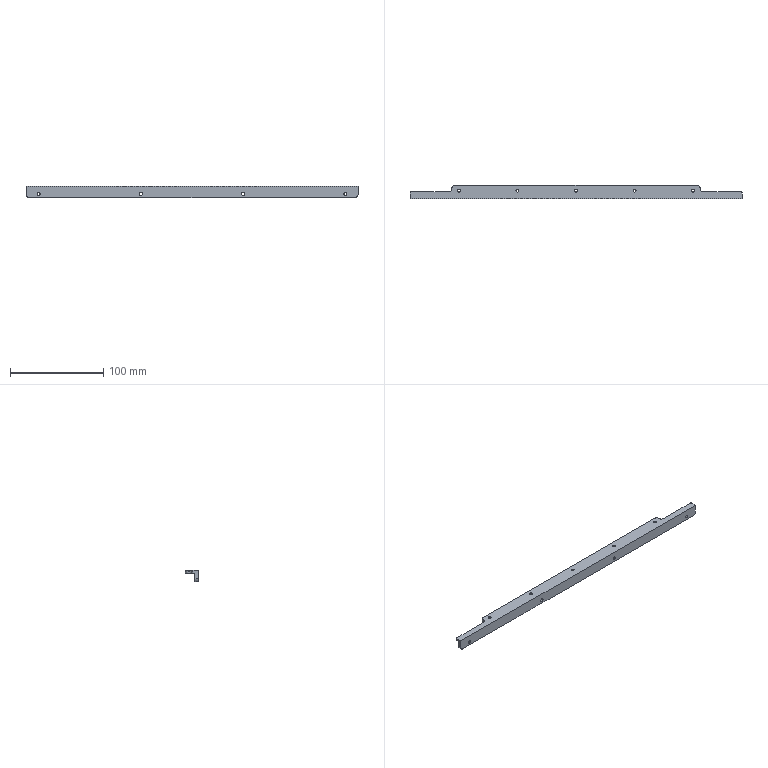Part | 1 solid | 48 faces | box 356.96 x 14 x 12 mm | volume 25600 mm3 | cylinder 26 | plane 12 | cone 10 | commonest cylinder face diameters 3.2 x10 3.3 x8 6 x6 2 x2
STEP:
#1=CARTESIAN_POINT('',(165.,4.,-6.35));
#2=VERTEX_POINT('',#1);
#3=CARTESIAN_POINT('',(165.,0.,-6.35));
#4=VERTEX_POINT('',#3);
#5=CARTESIAN_POINT('',(165.,0.,-6.35));
#6=DIRECTION('',(0.,-1.,0.));
#7=VECTOR('',#6,1000.);
#8=LINE('',#5,#7);
#9=EDGE_CURVE('',#2,#4,#8,.T.);
#10=ORIENTED_EDGE('',*,*,#9,.F.);
#11=CARTESIAN_POINT('',(165.,4.,-9.65));
#12=VERTEX_POINT('',#11);
#13=CARTESIAN_POINT('',(165.,4.,-8.));
#14=DIRECTION('',(0.,-1.,0.));
#15=DIRECTION('',(0.,0.,-1.));
#16=AXIS2_PLACEMENT_3D('',#13,#14,#15);
#17=CIRCLE('',#16,1.65);
#18=EDGE_CURVE('',#12,#2,#17,.T.);
#19=ORIENTED_EDGE('',*,*,#18,.F.);
#20=CARTESIAN_POINT('',(165.,0.,-9.65));
#21=VERTEX_POINT('',#20);
#22=CARTESIAN_POINT('',(165.,0.,-9.65));
#23=DIRECTION('',(0.,-1.,0.));
#24=VECTOR('',#23,1000.);
#25=LINE('',#22,#24);
#26=EDGE_CURVE('',#12,#21,#25,.T.);
#27=ORIENTED_EDGE('',*,*,#26,.T.);
#28=CARTESIAN_POINT('',(165.,0.,-8.));
#29=DIRECTION('',(0.,-1.,0.));
#30=DIRECTION('',(0.,0.,-1.));
#31=AXIS2_PLACEMENT_3D('',#28,#29,#30);
#32=CIRCLE('',#31,1.65);
#33=EDGE_CURVE('',#21,#4,#32,.T.);
#34=ORIENTED_EDGE('',*,*,#33,.T.);
#35=EDGE_LOOP('',(#10,#19,#27,#34));
#36=FACE_BOUND('',#35,.T.);
#37=CARTESIAN_POINT('',(165.,0.,-8.));
#38=DIRECTION('',(0.,-1.,0.));
#39=DIRECTION('',(0.,0.,-1.));
#40=AXIS2_PLACEMENT_3D('',#37,#38,#39);
#41=CYLINDRICAL_SURFACE('',#40,1.65);
#42=ADVANCED_FACE('',(#36),#41,.F.);
#43=CARTESIAN_POINT('',(55.,4.,-6.35));
#44=VERTEX_POINT('',#43);
#45=CARTESIAN_POINT('',(55.,0.,-6.35));
#46=VERTEX_POINT('',#45);
#47=CARTESIAN_POINT('',(55.,0.,-6.35));
#48=DIRECTION('',(0.,-1.,0.));
#49=VECTOR('',#48,1000.);
#50=LINE('',#47,#49);
#51=EDGE_CURVE('',#44,#46,#50,.T.);
#52=ORIENTED_EDGE('',*,*,#51,.F.);
#53=CARTESIAN_POINT('',(55.,4.,-9.65));
#54=VERTEX_POINT('',#53);
#55=CARTESIAN_POINT('',(55.,4.,-8.));
#56=DIRECTION('',(0.,-1.,0.));
#57=DIRECTION('',(0.,0.,-1.));
#58=AXIS2_PLACEMENT_3D('',#55,#56,#57);
#59=CIRCLE('',#58,1.65);
#60=EDGE_CURVE('',#54,#44,#59,.T.);
#61=ORIENTED_EDGE('',*,*,#60,.F.);
#62=CARTESIAN_POINT('',(55.,0.,-9.65));
#63=VERTEX_POINT('',#62);
#64=CARTESIAN_POINT('',(55.,0.,-9.65));
#65=DIRECTION('',(0.,-1.,0.));
#66=VECTOR('',#65,1000.);
#67=LINE('',#64,#66);
#68=EDGE_CURVE('',#54,#63,#67,.T.);
#69=ORIENTED_EDGE('',*,*,#68,.T.);
#70=CARTESIAN_POINT('',(55.,0.,-8.));
#71=DIRECTION('',(0.,-1.,0.));
#72=DIRECTION('',(0.,0.,-1.));
#73=AXIS2_PLACEMENT_3D('',#70,#71,#72);
#74=CIRCLE('',#73,1.65);
#75=EDGE_CURVE('',#63,#46,#74,.T.);
#76=ORIENTED_EDGE('',*,*,#75,.T.);
#77=EDGE_LOOP('',(#52,#61,#69,#76));
#78=FACE_BOUND('',#77,.T.);
#79=CARTESIAN_POINT('',(55.,0.,-8.));
#80=DIRECTION('',(0.,-1.,0.));
#81=DIRECTION('',(0.,0.,-1.));
#82=AXIS2_PLACEMENT_3D('',#79,#80,#81);
#83=CYLINDRICAL_SURFACE('',#82,1.65);
#84=ADVANCED_FACE('',(#78),#83,.F.);
#85=CARTESIAN_POINT('',(-55.,4.,-6.35));
#86=VERTEX_POINT('',#85);
#87=CARTESIAN_POINT('',(-55.,0.,-6.35));
#88=VERTEX_POINT('',#87);
#89=CARTESIAN_POINT('',(-55.,0.,-6.35));
#90=DIRECTION('',(0.,-1.,0.));
#91=VECTOR('',#90,1000.);
#92=LINE('',#89,#91);
#93=EDGE_CURVE('',#86,#88,#92,.T.);
#94=ORIENTED_EDGE('',*,*,#93,.F.);
#95=CARTESIAN_POINT('',(-55.,4.,-9.65));
#96=VERTEX_POINT('',#95);
#97=CARTESIAN_POINT('',(-55.,4.,-8.));
#98=DIRECTION('',(0.,-1.,0.));
#99=DIRECTION('',(0.,0.,-1.));
#100=AXIS2_PLACEMENT_3D('',#97,#98,#99);
#101=CIRCLE('',#100,1.65);
#102=EDGE_CURVE('',#96,#86,#101,.T.);
#103=ORIENTED_EDGE('',*,*,#102,.F.);
#104=CARTESIAN_POINT('',(-55.,0.,-9.65));
#105=VERTEX_POINT('',#104);
#106=CARTESIAN_POINT('',(-55.,0.,-9.65));
#107=DIRECTION('',(0.,-1.,0.));
#108=VECTOR('',#107,1000.);
#109=LINE('',#106,#108);
#110=EDGE_CURVE('',#96,#105,#109,.T.);
#111=ORIENTED_EDGE('',*,*,#110,.T.);
#112=CARTESIAN_POINT('',(-55.,0.,-8.));
#113=DIRECTION('',(0.,-1.,0.));
#114=DIRECTION('',(0.,0.,-1.));
#115=AXIS2_PLACEMENT_3D('',#112,#113,#114);
#116=CIRCLE('',#115,1.65);
#117=EDGE_CURVE('',#105,#88,#116,.T.);
#118=ORIENTED_EDGE('',*,*,#117,.T.);
#119=EDGE_LOOP('',(#94,#103,#111,#118));
#120=FACE_BOUND('',#119,.T.);
#121=CARTESIAN_POINT('',(-55.,0.,-8.));
#122=DIRECTION('',(0.,-1.,0.));
#123=DIRECTION('',(0.,0.,-1.));
#124=AXIS2_PLACEMENT_3D('',#121,#122,#123);
#125=CYLINDRICAL_SURFACE('',#124,1.65);
#126=ADVANCED_FACE('',(#120),#125,.F.);
#127=CARTESIAN_POINT('',(-165.,4.,-6.35));
#128=VERTEX_POINT('',#127);
#129=CARTESIAN_POINT('',(-165.,0.,-6.35));
#130=VERTEX_POINT('',#129);
#131=CARTESIAN_POINT('',(-165.,0.,-6.35));
#132=DIRECTION('',(0.,-1.,0.));
#133=VECTOR('',#132,1000.);
#134=LINE('',#131,#133);
#135=EDGE_CURVE('',#128,#130,#134,.T.);
#136=ORIENTED_EDGE('',*,*,#135,.F.);
#137=CARTESIAN_POINT('',(-165.,4.,-9.65));
#138=VERTEX_POINT('',#137);
#139=CARTESIAN_POINT('',(-165.,4.,-8.));
#140=DIRECTION('',(0.,-1.,0.));
#141=DIRECTION('',(0.,0.,-1.));
#142=AXIS2_PLACEMENT_3D('',#139,#140,#141);
#143=CIRCLE('',#142,1.65);
#144=EDGE_CURVE('',#138,#128,#143,.T.);
#145=ORIENTED_EDGE('',*,*,#144,.F.);
#146=CARTESIAN_POINT('',(-165.,0.,-9.65));
#147=VERTEX_POINT('',#146);
#148=CARTESIAN_POINT('',(-165.,0.,-9.65));
#149=DIRECTION('',(0.,-1.,0.));
#150=VECTOR('',#149,1000.);
#151=LINE('',#148,#150);
#152=EDGE_CURVE('',#138,#147,#151,.T.);
#153=ORIENTED_EDGE('',*,*,#152,.T.);
#154=CARTESIAN_POINT('',(-165.,0.,-8.));
#155=DIRECTION('',(0.,-1.,0.));
#156=DIRECTION('',(0.,0.,-1.));
#157=AXIS2_PLACEMENT_3D('',#154,#155,#156);
#158=CIRCLE('',#157,1.65);
#159=EDGE_CURVE('',#147,#130,#158,.T.);
#160=ORIENTED_EDGE('',*,*,#159,.T.);
#161=EDGE_LOOP('',(#136,#145,#153,#160));
#162=FACE_BOUND('',#161,.T.);
#163=CARTESIAN_POINT('',(-165.,0.,-8.));
#164=DIRECTION('',(0.,-1.,0.));
#165=DIRECTION('',(0.,0.,-1.));
#166=AXIS2_PLACEMENT_3D('',#163,#164,#165);
#167=CYLINDRICAL_SURFACE('',#166,1.65);
#168=ADVANCED_FACE('',(#162),#167,.F.);
#169=CARTESIAN_POINT('',(126.,6.9,-1.45));
#170=VERTEX_POINT('',#169);
#171=CARTESIAN_POINT('',(126.,5.35,-3.));
#172=VERTEX_POINT('',#171);
#173=CARTESIAN_POINT('',(126.,5.35,-3.));
#174=DIRECTION('',(0.,-0.7071,-0.7071));
#175=VECTOR('',#174,1000.);
#176=LINE('',#173,#175);
#177=EDGE_CURVE('',#170,#172,#176,.T.);
#178=ORIENTED_EDGE('',*,*,#177,.F.);
#179=CARTESIAN_POINT('',(126.,10.1,-1.45));
#180=VERTEX_POINT('',#179);
#181=CARTESIAN_POINT('',(126.,8.5,-1.45));
#182=DIRECTION('',(0.,0.,-1.));
#183=DIRECTION('',(0.,1.,0.));
#184=AXIS2_PLACEMENT_3D('',#181,#182,#183);
#185=CIRCLE('',#184,1.6);
#186=EDGE_CURVE('',#180,#170,#185,.T.);
#187=ORIENTED_EDGE('',*,*,#186,.F.);
#188=CARTESIAN_POINT('',(126.,11.65,-3.));
#189=VERTEX_POINT('',#188);
#190=CARTESIAN_POINT('',(126.,11.65,-3.));
#191=DIRECTION('',(0.,0.7071,-0.7071));
#192=VECTOR('',#191,1000.);
#193=LINE('',#190,#192);
#194=EDGE_CURVE('',#180,#189,#193,.T.);
#195=ORIENTED_EDGE('',*,*,#194,.T.);
#196=CARTESIAN_POINT('',(126.,8.5,-3.));
#197=DIRECTION('',(0.,0.,-1.));
#198=DIRECTION('',(0.,1.,0.));
#199=AXIS2_PLACEMENT_3D('',#196,#197,#198);
#200=CIRCLE('',#199,3.15);
#201=EDGE_CURVE('',#189,#172,#200,.T.);
#202=ORIENTED_EDGE('',*,*,#201,.T.);
#203=EDGE_LOOP('',(#178,#187,#195,#202));
#204=FACE_BOUND('',#203,.T.);
#205=CARTESIAN_POINT('',(126.,8.5,-3.));
#206=DIRECTION('',(0.,0.,-1.));
#207=DIRECTION('',(0.,1.,0.));
#208=AXIS2_PLACEMENT_3D('',#205,#206,#207);
#209=CONICAL_SURFACE('',#208,3.15,0.7854);
#210=ADVANCED_FACE('',(#204),#209,.F.);
#211=CARTESIAN_POINT('',(126.,6.9,0.));
#212=VERTEX_POINT('',#211);
#213=CARTESIAN_POINT('',(126.,6.9,-3.));
#214=DIRECTION('',(0.,0.,-1.));
#215=VECTOR('',#214,1000.);
#216=LINE('',#213,#215);
#217=EDGE_CURVE('',#212,#170,#216,.T.);
#218=ORIENTED_EDGE('',*,*,#217,.F.);
#219=CARTESIAN_POINT('',(126.,10.1,0.));
#220=VERTEX_POINT('',#219);
#221=CARTESIAN_POINT('',(126.,8.5,0.));
#222=DIRECTION('',(0.,0.,-1.));
#223=DIRECTION('',(-1.,0.,0.));
#224=AXIS2_PLACEMENT_3D('',#221,#222,#223);
#225=CIRCLE('',#224,1.6);
#226=EDGE_CURVE('',#220,#212,#225,.T.);
#227=ORIENTED_EDGE('',*,*,#226,.F.);
#228=CARTESIAN_POINT('',(126.,10.1,-3.));
#229=DIRECTION('',(0.,0.,-1.));
#230=VECTOR('',#229,1000.);
#231=LINE('',#228,#230);
#232=EDGE_CURVE('',#220,#180,#231,.T.);
#233=ORIENTED_EDGE('',*,*,#232,.T.);
#234=ORIENTED_EDGE('',*,*,#186,.T.);
#235=EDGE_LOOP('',(#218,#227,#233,#234));
#236=FACE_BOUND('',#235,.T.);
#237=CARTESIAN_POINT('',(126.,8.5,-3.));
#238=DIRECTION('',(0.,0.,-1.));
#239=DIRECTION('',(0.,1.,0.));
#240=AXIS2_PLACEMENT_3D('',#237,#238,#239);
#241=CYLINDRICAL_SURFACE('',#240,1.6);
#242=ADVANCED_FACE('',(#236),#241,.F.);
#243=CARTESIAN_POINT('',(63.,6.9,-1.45));
#244=VERTEX_POINT('',#243);
#245=CARTESIAN_POINT('',(63.,5.35,-3.));
#246=VERTEX_POINT('',#245);
#247=CARTESIAN_POINT('',(63.,5.35,-3.));
#248=DIRECTION('',(0.,-0.7071,-0.7071));
#249=VECTOR('',#248,1000.);
#250=LINE('',#247,#249);
#251=EDGE_CURVE('',#244,#246,#250,.T.);
#252=ORIENTED_EDGE('',*,*,#251,.F.);
#253=CARTESIAN_POINT('',(63.,10.1,-1.45));
#254=VERTEX_POINT('',#253);
#255=CARTESIAN_POINT('',(63.,8.5,-1.45));
#256=DIRECTION('',(0.,0.,-1.));
#257=DIRECTION('',(0.,1.,0.));
#258=AXIS2_PLACEMENT_3D('',#255,#256,#257);
#259=CIRCLE('',#258,1.6);
#260=EDGE_CURVE('',#254,#244,#259,.T.);
#261=ORIENTED_EDGE('',*,*,#260,.F.);
#262=CARTESIAN_POINT('',(63.,11.65,-3.));
#263=VERTEX_POINT('',#262);
#264=CARTESIAN_POINT('',(63.,11.65,-3.));
#265=DIRECTION('',(0.,0.7071,-0.7071));
#266=VECTOR('',#265,1000.);
#267=LINE('',#264,#266);
#268=EDGE_CURVE('',#254,#263,#267,.T.);
#269=ORIENTED_EDGE('',*,*,#268,.T.);
#270=CARTESIAN_POINT('',(63.,8.5,-3.));
#271=DIRECTION('',(0.,0.,-1.));
#272=DIRECTION('',(0.,1.,0.));
#273=AXIS2_PLACEMENT_3D('',#270,#271,#272);
#274=CIRCLE('',#273,3.15);
#275=EDGE_CURVE('',#263,#246,#274,.T.);
#276=ORIENTED_EDGE('',*,*,#275,.T.);
#277=EDGE_LOOP('',(#252,#261,#269,#276));
#278=FACE_BOUND('',#277,.T.);
#279=CARTESIAN_POINT('',(63.,8.5,-3.));
#280=DIRECTION('',(0.,0.,-1.));
#281=DIRECTION('',(0.,1.,0.));
#282=AXIS2_PLACEMENT_3D('',#279,#280,#281);
#283=CONICAL_SURFACE('',#282,3.15,0.7854);
#284=ADVANCED_FACE('',(#278),#283,.F.);
#285=CARTESIAN_POINT('',(63.,6.9,0.));
#286=VERTEX_POINT('',#285);
#287=CARTESIAN_POINT('',(63.,6.9,-3.));
#288=DIRECTION('',(0.,0.,-1.));
#289=VECTOR('',#288,1000.);
#290=LINE('',#287,#289);
#291=EDGE_CURVE('',#286,#244,#290,.T.);
#292=ORIENTED_EDGE('',*,*,#291,.F.);
#293=CARTESIAN_POINT('',(63.,10.1,0.));
#294=VERTEX_POINT('',#293);
#295=CARTESIAN_POINT('',(63.,8.5,0.));
#296=DIRECTION('',(0.,0.,-1.));
#297=DIRECTION('',(-1.,0.,0.));
#298=AXIS2_PLACEMENT_3D('',#295,#296,#297);
#299=CIRCLE('',#298,1.6);
#300=EDGE_CURVE('',#294,#286,#299,.T.);
#301=ORIENTED_EDGE('',*,*,#300,.F.);
#302=CARTESIAN_POINT('',(63.,10.1,-3.));
#303=DIRECTION('',(0.,0.,-1.));
#304=VECTOR('',#303,1000.);
#305=LINE('',#302,#304);
#306=EDGE_CURVE('',#294,#254,#305,.T.);
#307=ORIENTED_EDGE('',*,*,#306,.T.);
#308=ORIENTED_EDGE('',*,*,#260,.T.);
#309=EDGE_LOOP('',(#292,#301,#307,#308));
#310=FACE_BOUND('',#309,.T.);
#311=CARTESIAN_POINT('',(63.,8.5,-3.));
#312=DIRECTION('',(0.,0.,-1.));
#313=DIRECTION('',(0.,1.,0.));
#314=AXIS2_PLACEMENT_3D('',#311,#312,#313);
#315=CYLINDRICAL_SURFACE('',#314,1.6);
#316=ADVANCED_FACE('',(#310),#315,.F.);
#317=CARTESIAN_POINT('',(0.,6.9,-1.45));
#318=VERTEX_POINT('',#317);
#319=CARTESIAN_POINT('',(0.,5.35,-3.));
#320=VERTEX_POINT('',#319);
#321=CARTESIAN_POINT('',(0.,5.35,-3.));
#322=DIRECTION('',(0.,-0.7071,-0.7071));
#323=VECTOR('',#322,1000.);
#324=LINE('',#321,#323);
#325=EDGE_CURVE('',#318,#320,#324,.T.);
#326=ORIENTED_EDGE('',*,*,#325,.F.);
#327=CARTESIAN_POINT('',(0.,10.1,-1.45));
#328=VERTEX_POINT('',#327);
#329=CARTESIAN_POINT('',(0.,8.5,-1.45));
#330=DIRECTION('',(0.,0.,-1.));
#331=DIRECTION('',(0.,1.,0.));
#332=AXIS2_PLACEMENT_3D('',#329,#330,#331);
#333=CIRCLE('',#332,1.6);
#334=EDGE_CURVE('',#328,#318,#333,.T.);
#335=ORIENTED_EDGE('',*,*,#334,.F.);
#336=CARTESIAN_POINT('',(0.,11.65,-3.));
#337=VERTEX_POINT('',#336);
#338=CARTESIAN_POINT('',(0.,11.65,-3.));
#339=DIRECTION('',(0.,0.7071,-0.7071));
#340=VECTOR('',#339,1000.);
#341=LINE('',#338,#340);
#342=EDGE_CURVE('',#328,#337,#341,.T.);
#343=ORIENTED_EDGE('',*,*,#342,.T.);
#344=CARTESIAN_POINT('',(0.,8.5,-3.));
#345=DIRECTION('',(0.,0.,-1.));
#346=DIRECTION('',(0.,1.,0.));
#347=AXIS2_PLACEMENT_3D('',#344,#345,#346);
#348=CIRCLE('',#347,3.15);
#349=EDGE_CURVE('',#337,#320,#348,.T.);
#350=ORIENTED_EDGE('',*,*,#349,.T.);
#351=EDGE_LOOP('',(#326,#335,#343,#350));
#352=FACE_BOUND('',#351,.T.);
#353=CARTESIAN_POINT('',(0.,8.5,-3.));
#354=DIRECTION('',(0.,0.,-1.));
#355=DIRECTION('',(0.,1.,0.));
#356=AXIS2_PLACEMENT_3D('',#353,#354,#355);
#357=CONICAL_SURFACE('',#356,3.15,0.7854);
#358=ADVANCED_FACE('',(#352),#357,.F.);
#359=CARTESIAN_POINT('',(0.,6.9,0.));
#360=VERTEX_POINT('',#359);
#361=CARTESIAN_POINT('',(0.,6.9,-3.));
#362=DIRECTION('',(0.,0.,-1.));
#363=VECTOR('',#362,1000.);
#364=LINE('',#361,#363);
#365=EDGE_CURVE('',#360,#318,#364,.T.);
#366=ORIENTED_EDGE('',*,*,#365,.F.);
#367=CARTESIAN_POINT('',(0.,10.1,0.));
#368=VERTEX_POINT('',#367);
#369=CARTESIAN_POINT('',(0.,8.5,0.));
#370=DIRECTION('',(0.,0.,-1.));
#371=DIRECTION('',(-1.,0.,0.));
#372=AXIS2_PLACEMENT_3D('',#369,#370,#371);
#373=CIRCLE('',#372,1.6);
#374=EDGE_CURVE('',#368,#360,#373,.T.);
#375=ORIENTED_EDGE('',*,*,#374,.F.);
#376=CARTESIAN_POINT('',(0.,10.1,-3.));
#377=DIRECTION('',(0.,0.,-1.));
#378=VECTOR('',#377,1000.);
#379=LINE('',#376,#378);
#380=EDGE_CURVE('',#368,#328,#379,.T.);
#381=ORIENTED_EDGE('',*,*,#380,.T.);
#382=ORIENTED_EDGE('',*,*,#334,.T.);
#383=EDGE_LOOP('',(#366,#375,#381,#382));
#384=FACE_BOUND('',#383,.T.);
#385=CARTESIAN_POINT('',(0.,8.5,-3.));
#386=DIRECTION('',(0.,0.,-1.));
#387=DIRECTION('',(0.,1.,0.));
#388=AXIS2_PLACEMENT_3D('',#385,#386,#387);
#389=CYLINDRICAL_SURFACE('',#388,1.6);
#390=ADVANCED_FACE('',(#384),#389,.F.);
#391=CARTESIAN_POINT('',(-63.,6.9,-1.45));
#392=VERTEX_POINT('',#391);
#393=CARTESIAN_POINT('',(-63.,5.35,-3.));
#394=VERTEX_POINT('',#393);
#395=CARTESIAN_POINT('',(-63.,5.35,-3.));
#396=DIRECTION('',(0.,-0.7071,-0.7071));
#397=VECTOR('',#396,1000.);
#398=LINE('',#395,#397);
#399=EDGE_CURVE('',#392,#394,#398,.T.);
#400=ORIENTED_EDGE('',*,*,#399,.F.);
#401=CARTESIAN_POINT('',(-63.,10.1,-1.45));
#402=VERTEX_POINT('',#401);
#403=CARTESIAN_POINT('',(-63.,8.5,-1.45));
#404=DIRECTION('',(0.,0.,-1.));
#405=DIRECTION('',(0.,1.,0.));
#406=AXIS2_PLACEMENT_3D('',#403,#404,#405);
#407=CIRCLE('',#406,1.6);
#408=EDGE_CURVE('',#402,#392,#407,.T.);
#409=ORIENTED_EDGE('',*,*,#408,.F.);
#410=CARTESIAN_POINT('',(-63.,11.65,-3.));
#411=VERTEX_POINT('',#410);
#412=CARTESIAN_POINT('',(-63.,11.65,-3.));
#413=DIRECTION('',(0.,0.7071,-0.7071));
#414=VECTOR('',#413,1000.);
#415=LINE('',#412,#414);
#416=EDGE_CURVE('',#402,#411,#415,.T.);
#417=ORIENTED_EDGE('',*,*,#416,.T.);
#418=CARTESIAN_POINT('',(-63.,8.5,-3.));
#419=DIRECTION('',(0.,0.,-1.));
#420=DIRECTION('',(0.,1.,0.));
#421=AXIS2_PLACEMENT_3D('',#418,#419,#420);
#422=CIRCLE('',#421,3.15);
#423=EDGE_CURVE('',#411,#394,#422,.T.);
#424=ORIENTED_EDGE('',*,*,#423,.T.);
#425=EDGE_LOOP('',(#400,#409,#417,#424));
#426=FACE_BOUND('',#425,.T.);
#427=CARTESIAN_POINT('',(-63.,8.5,-3.));
#428=DIRECTION('',(0.,0.,-1.));
#429=DIRECTION('',(0.,1.,0.));
#430=AXIS2_PLACEMENT_3D('',#427,#428,#429);
#431=CONICAL_SURFACE('',#430,3.15,0.7854);
#432=ADVANCED_FACE('',(#426),#431,.F.);
#433=CARTESIAN_POINT('',(-63.,6.9,0.));
#434=VERTEX_POINT('',#433);
#435=CARTESIAN_POINT('',(-63.,6.9,-3.));
#436=DIRECTION('',(0.,0.,-1.));
#437=VECTOR('',#436,1000.);
#438=LINE('',#435,#437);
#439=EDGE_CURVE('',#434,#392,#438,.T.);
#440=ORIENTED_EDGE('',*,*,#439,.F.);
#441=CARTESIAN_POINT('',(-63.,10.1,0.));
#442=VERTEX_POINT('',#441);
#443=CARTESIAN_POINT('',(-63.,8.5,0.));
#444=DIRECTION('',(0.,0.,-1.));
#445=DIRECTION('',(-1.,0.,0.));
#446=AXIS2_PLACEMENT_3D('',#443,#444,#445);
#447=CIRCLE('',#446,1.6);
#448=EDGE_CURVE('',#442,#434,#447,.T.);
#449=ORIENTED_EDGE('',*,*,#448,.F.);
#450=CARTESIAN_POINT('',(-63.,10.1,-3.));
#451=DIRECTION('',(0.,0.,-1.));
#452=VECTOR('',#451,1000.);
#453=LINE('',#450,#452);
#454=EDGE_CURVE('',#442,#402,#453,.T.);
#455=ORIENTED_EDGE('',*,*,#454,.T.);
#456=ORIENTED_EDGE('',*,*,#408,.T.);
#457=EDGE_LOOP('',(#440,#449,#455,#456));
#458=FACE_BOUND('',#457,.T.);
#459=CARTESIAN_POINT('',(-63.,8.5,-3.));
#460=DIRECTION('',(0.,0.,-1.));
#461=DIRECTION('',(0.,1.,0.));
#462=AXIS2_PLACEMENT_3D('',#459,#460,#461);
#463=CYLINDRICAL_SURFACE('',#462,1.6);
#464=ADVANCED_FACE('',(#458),#463,.F.);
#465=CARTESIAN_POINT('',(-126.,6.9,-1.45));
#466=VERTEX_POINT('',#465);
#467=CARTESIAN_POINT('',(-126.,5.35,-3.));
#468=VERTEX_POINT('',#467);
#469=CARTESIAN_POINT('',(-126.,5.35,-3.));
#470=DIRECTION('',(0.,-0.7071,-0.7071));
#471=VECTOR('',#470,1000.);
#472=LINE('',#469,#471);
#473=EDGE_CURVE('',#466,#468,#472,.T.);
#474=ORIENTED_EDGE('',*,*,#473,.F.);
#475=CARTESIAN_POINT('',(-126.,10.1,-1.45));
#476=VERTEX_POINT('',#475);
#477=CARTESIAN_POINT('',(-126.,8.5,-1.45));
#478=DIRECTION('',(0.,0.,-1.));
#479=DIRECTION('',(0.,1.,0.));
#480=AXIS2_PLACEMENT_3D('',#477,#478,#479);
#481=CIRCLE('',#480,1.6);
#482=EDGE_CURVE('',#476,#466,#481,.T.);
#483=ORIENTED_EDGE('',*,*,#482,.F.);
#484=CARTESIAN_POINT('',(-126.,11.65,-3.));
#485=VERTEX_POINT('',#484);
#486=CARTESIAN_POINT('',(-126.,11.65,-3.));
#487=DIRECTION('',(0.,0.7071,-0.7071));
#488=VECTOR('',#487,1000.);
#489=LINE('',#486,#488);
#490=EDGE_CURVE('',#476,#485,#489,.T.);
#491=ORIENTED_EDGE('',*,*,#490,.T.);
#492=CARTESIAN_POINT('',(-126.,8.5,-3.));
#493=DIRECTION('',(0.,0.,-1.));
#494=DIRECTION('',(0.,1.,0.));
#495=AXIS2_PLACEMENT_3D('',#492,#493,#494);
#496=CIRCLE('',#495,3.15);
#497=EDGE_CURVE('',#485,#468,#496,.T.);
#498=ORIENTED_EDGE('',*,*,#497,.T.);
#499=EDGE_LOOP('',(#474,#483,#491,#498));
#500=FACE_BOUND('',#499,.T.);
#501=CARTESIAN_POINT('',(-126.,8.5,-3.));
#502=DIRECTION('',(0.,0.,-1.));
#503=DIRECTION('',(0.,1.,0.));
#504=AXIS2_PLACEMENT_3D('',#501,#502,#503);
#505=CONICAL_SURFACE('',#504,3.15,0.7854);
#506=ADVANCED_FACE('',(#500),#505,.F.);
#507=CARTESIAN_POINT('',(-126.,6.9,0.));
#508=VERTEX_POINT('',#507);
#509=CARTESIAN_POINT('',(-126.,6.9,-3.));
#510=DIRECTION('',(0.,0.,-1.));
#511=VECTOR('',#510,1000.);
#512=LINE('',#509,#511);
#513=EDGE_CURVE('',#508,#466,#512,.T.);
#514=ORIENTED_EDGE('',*,*,#513,.F.);
#515=CARTESIAN_POINT('',(-126.,10.1,0.));
#516=VERTEX_POINT('',#515);
#517=CARTESIAN_POINT('',(-126.,8.5,0.));
#518=DIRECTION('',(0.,0.,-1.));
#519=DIRECTION('',(-1.,0.,0.));
#520=AXIS2_PLACEMENT_3D('',#517,#518,#519);
#521=CIRCLE('',#520,1.6);
#522=EDGE_CURVE('',#516,#508,#521,.T.);
#523=ORIENTED_EDGE('',*,*,#522,.F.);
#524=CARTESIAN_POINT('',(-126.,10.1,-3.));
#525=DIRECTION('',(0.,0.,-1.));
#526=VECTOR('',#525,1000.);
#527=LINE('',#524,#526);
#528=EDGE_CURVE('',#516,#476,#527,.T.);
#529=ORIENTED_EDGE('',*,*,#528,.T.);
#530=ORIENTED_EDGE('',*,*,#482,.T.);
#531=EDGE_LOOP('',(#514,#523,#529,#530));
#532=FACE_BOUND('',#531,.T.);
#533=CARTESIAN_POINT('',(-126.,8.5,-3.));
#534=DIRECTION('',(0.,0.,-1.));
#535=DIRECTION('',(0.,1.,0.));
#536=AXIS2_PLACEMENT_3D('',#533,#534,#535);
#537=CYLINDRICAL_SURFACE('',#536,1.6);
#538=ADVANCED_FACE('',(#532),#537,.F.);
#539=CARTESIAN_POINT('',(177.48,7.,-3.));
#540=VERTEX_POINT('',#539);
#541=CARTESIAN_POINT('',(178.48,6.,-3.));
#542=VERTEX_POINT('',#541);
#543=CARTESIAN_POINT('',(177.48,6.,-3.));
#544=DIRECTION('',(0.,0.,-1.));
#545=DIRECTION('',(0.,-1.,0.));
#546=AXIS2_PLACEMENT_3D('',#543,#544,#545);
#547=CIRCLE('',#546,1.);
#548=EDGE_CURVE('',#540,#542,#547,.T.);
#549=ORIENTED_EDGE('',*,*,#548,.F.);
#550=CARTESIAN_POINT('',(177.48,7.,0.));
#551=VERTEX_POINT('',#550);
#552=CARTESIAN_POINT('',(177.48,7.,-12.001));
#553=DIRECTION('',(0.,0.,-1.));
#554=VECTOR('',#553,1000.);
#555=LINE('',#552,#554);
#556=EDGE_CURVE('',#551,#540,#555,.T.);
#557=ORIENTED_EDGE('',*,*,#556,.F.);
#558=CARTESIAN_POINT('',(178.48,6.,0.));
#559=VERTEX_POINT('',#558);
#560=CARTESIAN_POINT('',(177.48,6.,0.));
#561=DIRECTION('',(0.,0.,1.));
#562=DIRECTION('',(-1.,0.,0.));
#563=AXIS2_PLACEMENT_3D('',#560,#561,#562);
#564=CIRCLE('',#563,1.);
#565=EDGE_CURVE('',#559,#551,#564,.T.);
#566=ORIENTED_EDGE('',*,*,#565,.F.);
#567=CARTESIAN_POINT('',(178.48,6.,0.));
#568=DIRECTION('',(0.,0.,1.));
#569=VECTOR('',#568,1000.);
#570=LINE('',#567,#569);
#571=EDGE_CURVE('',#542,#559,#570,.T.);
#572=ORIENTED_EDGE('',*,*,#571,.F.);
#573=EDGE_LOOP('',(#549,#557,#566,#572));
#574=FACE_BOUND('',#573,.T.);
#575=CARTESIAN_POINT('',(177.48,6.,0.));
#576=DIRECTION('',(0.,0.,1.));
#577=DIRECTION('',(1.,0.,0.));
#578=AXIS2_PLACEMENT_3D('',#575,#576,#577);
#579=CYLINDRICAL_SURFACE('',#578,1.);
#580=ADVANCED_FACE('',(#574),#579,.T.);
#581=CARTESIAN_POINT('',(-178.48,6.,-3.));
#582=VERTEX_POINT('',#581);
#583=CARTESIAN_POINT('',(-177.48,7.,-3.));
#584=VERTEX_POINT('',#583);
#585=CARTESIAN_POINT('',(-177.48,6.,-3.));
#586=DIRECTION('',(0.,0.,-1.));
#587=DIRECTION('',(0.,-1.,0.));
#588=AXIS2_PLACEMENT_3D('',#585,#586,#587);
#589=CIRCLE('',#588,1.);
#590=EDGE_CURVE('',#582,#584,#589,.T.);
#591=ORIENTED_EDGE('',*,*,#590,.F.);
#592=CARTESIAN_POINT('',(-178.48,6.,0.));
#593=VERTEX_POINT('',#592);
#594=CARTESIAN_POINT('',(-178.48,6.,-3.));
#595=DIRECTION('',(0.,0.,-1.));
#596=VECTOR('',#595,1000.);
#597=LINE('',#594,#596);
#598=EDGE_CURVE('',#593,#582,#597,.T.);
#599=ORIENTED_EDGE('',*,*,#598,.F.);
#600=CARTESIAN_POINT('',(-177.48,7.,0.));
#601=VERTEX_POINT('',#600);
#602=CARTESIAN_POINT('',(-177.48,6.,0.));
#603=DIRECTION('',(0.,0.,1.));
#604=DIRECTION('',(-1.,0.,0.));
#605=AXIS2_PLACEMENT_3D('',#602,#603,#604);
#606=CIRCLE('',#605,1.);
#607=EDGE_CURVE('',#601,#593,#606,.T.);
#608=ORIENTED_EDGE('',*,*,#607,.F.);
#609=CARTESIAN_POINT('',(-177.48,7.,0.));
#610=DIRECTION('',(0.,0.,1.));
#611=VECTOR('',#610,1000.);
#612=LINE('',#609,#611);
#613=EDGE_CURVE('',#584,#601,#612,.T.);
#614=ORIENTED_EDGE('',*,*,#613,.F.);
#615=EDGE_LOOP('',(#591,#599,#608,#614));
#616=FACE_BOUND('',#615,.T.);
#617=CARTESIAN_POINT('',(-177.48,6.,-12.001));
#618=DIRECTION('',(0.,0.,-1.));
#619=DIRECTION('',(-1.,0.,0.));
#620=AXIS2_PLACEMENT_3D('',#617,#618,#619);
#621=CYLINDRICAL_SURFACE('',#620,1.);
#622=ADVANCED_FACE('',(#616),#621,.T.);
#623=CARTESIAN_POINT('',(-133.5,11.,-3.));
#624=VERTEX_POINT('',#623);
#625=CARTESIAN_POINT('',(-130.5,14.,-3.));
#626=VERTEX_POINT('',#625);
#627=CARTESIAN_POINT('',(-130.5,11.,-3.));
#628=DIRECTION('',(0.,0.,-1.));
#629=DIRECTION('',(0.,-1.,0.));
#630=AXIS2_PLACEMENT_3D('',#627,#628,#629);
#631=CIRCLE('',#630,3.);
#632=EDGE_CURVE('',#624,#626,#631,.T.);
#633=ORIENTED_EDGE('',*,*,#632,.F.);
#634=CARTESIAN_POINT('',(-133.5,11.,0.));
#635=VERTEX_POINT('',#634);
#636=CARTESIAN_POINT('',(-133.5,11.,-12.001));
#637=DIRECTION('',(0.,0.,-1.));
#638=VECTOR('',#637,1000.);
#639=LINE('',#636,#638);
#640=EDGE_CURVE('',#635,#624,#639,.T.);
#641=ORIENTED_EDGE('',*,*,#640,.F.);
#642=CARTESIAN_POINT('',(-130.5,14.,0.));
#643=VERTEX_POINT('',#642);
#644=CARTESIAN_POINT('',(-130.5,11.,0.));
#645=DIRECTION('',(0.,0.,1.));
#646=DIRECTION('',(-1.,0.,0.));
#647=AXIS2_PLACEMENT_3D('',#644,#645,#646);
#648=CIRCLE('',#647,3.);
#649=EDGE_CURVE('',#643,#635,#648,.T.);
#650=ORIENTED_EDGE('',*,*,#649,.F.);
#651=CARTESIAN_POINT('',(-130.5,14.,0.));
#652=DIRECTION('',(0.,0.,1.));
#653=VECTOR('',#652,1000.);
#654=LINE('',#651,#653);
#655=EDGE_CURVE('',#626,#643,#654,.T.);
#656=ORIENTED_EDGE('',*,*,#655,.F.);
#657=EDGE_LOOP('',(#633,#641,#650,#656));
#658=FACE_BOUND('',#657,.T.);
#659=CARTESIAN_POINT('',(-130.5,11.,0.));
#660=DIRECTION('',(0.,0.,1.));
#661=DIRECTION('',(1.,0.,0.));
#662=AXIS2_PLACEMENT_3D('',#659,#660,#661);
#663=CYLINDRICAL_SURFACE('',#662,3.);
#664=ADVANCED_FACE('',(#658),#663,.T.);
#665=CARTESIAN_POINT('',(-136.5,7.,-3.));
#666=VERTEX_POINT('',#665);
#667=CARTESIAN_POINT('',(-133.5,10.,-3.));
#668=VERTEX_POINT('',#667);
#669=CARTESIAN_POINT('',(-136.5,10.,-3.));
#670=DIRECTION('',(0.,0.,1.));
#671=DIRECTION('',(0.,-1.,0.));
#672=AXIS2_PLACEMENT_3D('',#669,#670,#671);
#673=CIRCLE('',#672,3.);
#674=EDGE_CURVE('',#666,#668,#673,.T.);
#675=ORIENTED_EDGE('',*,*,#674,.F.);
#676=CARTESIAN_POINT('',(-136.5,7.,0.));
#677=VERTEX_POINT('',#676);
#678=CARTESIAN_POINT('',(-136.5,7.,-3.));
#679=DIRECTION('',(0.,0.,-1.));
#680=VECTOR('',#679,1000.);
#681=LINE('',#678,#680);
#682=EDGE_CURVE('',#677,#666,#681,.T.);
#683=ORIENTED_EDGE('',*,*,#682,.F.);
#684=CARTESIAN_POINT('',(-133.5,10.,0.));
#685=VERTEX_POINT('',#684);
#686=CARTESIAN_POINT('',(-136.5,10.,0.));
#687=DIRECTION('',(0.,0.,-1.));
#688=DIRECTION('',(-1.,0.,0.));
#689=AXIS2_PLACEMENT_3D('',#686,#687,#688);
#690=CIRCLE('',#689,3.);
#691=EDGE_CURVE('',#685,#677,#690,.T.);
#692=ORIENTED_EDGE('',*,*,#691,.F.);
#693=CARTESIAN_POINT('',(-133.5,10.,0.));
#694=DIRECTION('',(0.,0.,1.));
#695=VECTOR('',#694,1000.);
#696=LINE('',#693,#695);
#697=EDGE_CURVE('',#668,#685,#696,.T.);
#698=ORIENTED_EDGE('',*,*,#697,.F.);
#699=EDGE_LOOP('',(#675,#683,#692,#698));
#700=FACE_BOUND('',#699,.T.);
#701=CARTESIAN_POINT('',(-136.5,10.,-12.001));
#702=DIRECTION('',(0.,0.,-1.));
#703=DIRECTION('',(-1.,0.,0.));
#704=AXIS2_PLACEMENT_3D('',#701,#702,#703);
#705=CYLINDRICAL_SURFACE('',#704,3.);
#706=ADVANCED_FACE('',(#700),#705,.F.);
#707=CARTESIAN_POINT('',(-178.48,0.,-9.));
#708=VERTEX_POINT('',#707);
#709=CARTESIAN_POINT('',(-175.48,0.,-12.));
#710=VERTEX_POINT('',#709);
#711=CARTESIAN_POINT('',(-175.48,0.,-9.));
#712=DIRECTION('',(0.,-1.,0.));
#713=DIRECTION('',(0.,0.,1.));
#714=AXIS2_PLACEMENT_3D('',#711,#712,#713);
#715=CIRCLE('',#714,3.);
#716=EDGE_CURVE('',#708,#710,#715,.T.);
#717=ORIENTED_EDGE('',*,*,#716,.F.);
#718=CARTESIAN_POINT('',(-178.48,4.,-9.));
#719=VERTEX_POINT('',#718);
#720=CARTESIAN_POINT('',(-178.48,0.,-9.));
#721=DIRECTION('',(0.,-1.,0.));
#722=VECTOR('',#721,1000.);
#723=LINE('',#720,#722);
#724=EDGE_CURVE('',#719,#708,#723,.T.);
#725=ORIENTED_EDGE('',*,*,#724,.F.);
#726=CARTESIAN_POINT('',(-175.48,4.,-12.));
#727=VERTEX_POINT('',#726);
#728=CARTESIAN_POINT('',(-175.48,4.,-9.));
#729=DIRECTION('',(0.,1.,0.));
#730=DIRECTION('',(0.,0.,-1.));
#731=AXIS2_PLACEMENT_3D('',#728,#729,#730);
#732=CIRCLE('',#731,3.);
#733=EDGE_CURVE('',#727,#719,#732,.T.);
#734=ORIENTED_EDGE('',*,*,#733,.F.);
#735=CARTESIAN_POINT('',(-175.48,4.,-12.));
#736=DIRECTION('',(0.,1.,0.));
#737=VECTOR('',#736,1000.);
#738=LINE('',#735,#737);
#739=EDGE_CURVE('',#710,#727,#738,.T.);
#740=ORIENTED_EDGE('',*,*,#739,.F.);
#741=EDGE_LOOP('',(#717,#725,#734,#740));
#742=FACE_BOUND('',#741,.T.);
#743=CARTESIAN_POINT('',(-175.48,4.,-9.));
#744=DIRECTION('',(0.,-1.,0.));
#745=DIRECTION('',(0.,0.,-1.));
#746=AXIS2_PLACEMENT_3D('',#743,#744,#745);
#747=CYLINDRICAL_SURFACE('',#746,3.);
#748=ADVANCED_FACE('',(#742),#747,.T.);
#749=CARTESIAN_POINT('',(175.48,0.,-12.));
#750=VERTEX_POINT('',#749);
#751=CARTESIAN_POINT('',(178.48,0.,-9.));
#752=VERTEX_POINT('',#751);
#753=CARTESIAN_POINT('',(175.48,0.,-9.));
#754=DIRECTION('',(0.,-1.,0.));
#755=DIRECTION('',(0.,0.,1.));
#756=AXIS2_PLACEMENT_3D('',#753,#754,#755);
#757=CIRCLE('',#756,3.);
#758=EDGE_CURVE('',#750,#752,#757,.T.);
#759=ORIENTED_EDGE('',*,*,#758,.F.);
#760=CARTESIAN_POINT('',(175.48,4.,-12.));
#761=VERTEX_POINT('',#760);
#762=CARTESIAN_POINT('',(175.48,4.,-12.));
#763=DIRECTION('',(0.,-1.,0.));
#764=VECTOR('',#763,1000.);
#765=LINE('',#762,#764);
#766=EDGE_CURVE('',#761,#750,#765,.T.);
#767=ORIENTED_EDGE('',*,*,#766,.F.);
#768=CARTESIAN_POINT('',(178.48,4.,-9.));
#769=VERTEX_POINT('',#768);
#770=CARTESIAN_POINT('',(175.48,4.,-9.));
#771=DIRECTION('',(0.,1.,0.));
#772=DIRECTION('',(0.,0.,-1.));
#773=AXIS2_PLACEMENT_3D('',#770,#771,#772);
#774=CIRCLE('',#773,3.);
#775=EDGE_CURVE('',#769,#761,#774,.T.);
#776=ORIENTED_EDGE('',*,*,#775,.F.);
#777=CARTESIAN_POINT('',(178.48,0.,-9.));
#778=DIRECTION('',(0.,1.,0.));
#779=VECTOR('',#778,1000.);
#780=LINE('',#777,#779);
#781=EDGE_CURVE('',#752,#769,#780,.T.);
#782=ORIENTED_EDGE('',*,*,#781,.F.);
#783=EDGE_LOOP('',(#759,#767,#776,#782));
#784=FACE_BOUND('',#783,.T.);
#785=CARTESIAN_POINT('',(175.48,0.,-9.));
#786=DIRECTION('',(0.,1.,0.));
#787=DIRECTION('',(0.,0.,1.));
#788=AXIS2_PLACEMENT_3D('',#785,#786,#787);
#789=CYLINDRICAL_SURFACE('',#788,3.);
#790=ADVANCED_FACE('',(#784),#789,.T.);
#791=CARTESIAN_POINT('',(133.5,10.,-3.));
#792=VERTEX_POINT('',#791);
#793=CARTESIAN_POINT('',(136.5,7.,-3.));
#794=VERTEX_POINT('',#793);
#795=CARTESIAN_POINT('',(136.5,10.,-3.));
#796=DIRECTION('',(0.,0.,1.));
#797=DIRECTION('',(0.,-1.,0.));
#798=AXIS2_PLACEMENT_3D('',#795,#796,#797);
#799=CIRCLE('',#798,3.);
#800=EDGE_CURVE('',#792,#794,#799,.T.);
#801=ORIENTED_EDGE('',*,*,#800,.F.);
#802=CARTESIAN_POINT('',(133.5,10.,0.));
#803=VERTEX_POINT('',#802);
#804=CARTESIAN_POINT('',(133.5,10.,-3.));
#805=DIRECTION('',(0.,0.,-1.));
#806=VECTOR('',#805,1000.);
#807=LINE('',#804,#806);
#808=EDGE_CURVE('',#803,#792,#807,.T.);
#809=ORIENTED_EDGE('',*,*,#808,.F.);
#810=CARTESIAN_POINT('',(136.5,7.,0.));
#811=VERTEX_POINT('',#810);
#812=CARTESIAN_POINT('',(136.5,10.,0.));
#813=DIRECTION('',(0.,0.,-1.));
#814=DIRECTION('',(-1.,0.,0.));
#815=AXIS2_PLACEMENT_3D('',#812,#813,#814);
#816=CIRCLE('',#815,3.);
#817=EDGE_CURVE('',#811,#803,#816,.T.);
#818=ORIENTED_EDGE('',*,*,#817,.F.);
#819=CARTESIAN_POINT('',(136.5,7.,0.));
#820=DIRECTION('',(0.,0.,1.));
#821=VECTOR('',#820,1000.);
#822=LINE('',#819,#821);
#823=EDGE_CURVE('',#794,#811,#822,.T.);
#824=ORIENTED_EDGE('',*,*,#823,.F.);
#825=EDGE_LOOP('',(#801,#809,#818,#824));
#826=FACE_BOUND('',#825,.T.);
#827=CARTESIAN_POINT('',(136.5,10.,-12.001));
#828=DIRECTION('',(0.,0.,-1.));
#829=DIRECTION('',(-1.,0.,0.));
#830=AXIS2_PLACEMENT_3D('',#827,#828,#829);
#831=CYLINDRICAL_SURFACE('',#830,3.);
#832=ADVANCED_FACE('',(#826),#831,.F.);
#833=CARTESIAN_POINT('',(130.5,14.,-3.));
#834=VERTEX_POINT('',#833);
#835=CARTESIAN_POINT('',(133.5,11.,-3.));
#836=VERTEX_POINT('',#835);
#837=CARTESIAN_POINT('',(130.5,11.,-3.));
#838=DIRECTION('',(0.,0.,-1.));
#839=DIRECTION('',(0.,-1.,0.));
#840=AXIS2_PLACEMENT_3D('',#837,#838,#839);
#841=CIRCLE('',#840,3.);
#842=EDGE_CURVE('',#834,#836,#841,.T.);
#843=ORIENTED_EDGE('',*,*,#842,.F.);
#844=CARTESIAN_POINT('',(130.5,14.,0.));
#845=VERTEX_POINT('',#844);
#846=CARTESIAN_POINT('',(130.5,14.,0.));
#847=DIRECTION('',(0.,0.,-1.));
#848=VECTOR('',#847,1000.);
#849=LINE('',#846,#848);
#850=EDGE_CURVE('',#845,#834,#849,.T.);
#851=ORIENTED_EDGE('',*,*,#850,.F.);
#852=CARTESIAN_POINT('',(133.5,11.,0.));
#853=VERTEX_POINT('',#852);
#854=CARTESIAN_POINT('',(130.5,11.,0.));
#855=DIRECTION('',(0.,0.,1.));
#856=DIRECTION('',(-1.,0.,0.));
#857=AXIS2_PLACEMENT_3D('',#854,#855,#856);
#858=CIRCLE('',#857,3.);
#859=EDGE_CURVE('',#853,#845,#858,.T.);
#860=ORIENTED_EDGE('',*,*,#859,.F.);
#861=CARTESIAN_POINT('',(133.5,11.,-12.001));
#862=DIRECTION('',(0.,0.,1.));
#863=VECTOR('',#862,1000.);
#864=LINE('',#861,#863);
#865=EDGE_CURVE('',#836,#853,#864,.T.);
#866=ORIENTED_EDGE('',*,*,#865,.F.);
#867=EDGE_LOOP('',(#843,#851,#860,#866));
#868=FACE_BOUND('',#867,.T.);
#869=CARTESIAN_POINT('',(130.5,11.,-12.001));
#870=DIRECTION('',(0.,0.,1.));
#871=DIRECTION('',(1.,0.,0.));
#872=AXIS2_PLACEMENT_3D('',#869,#870,#871);
#873=CYLINDRICAL_SURFACE('',#872,3.);
#874=ADVANCED_FACE('',(#868),#873,.T.);
#875=CARTESIAN_POINT('',(133.5,14.,-3.));
#876=DIRECTION('',(0.,1.,0.));
#877=VECTOR('',#876,1000.);
#878=LINE('',#875,#877);
#879=EDGE_CURVE('',#792,#836,#878,.T.);
#880=ORIENTED_EDGE('',*,*,#879,.T.);
#881=ORIENTED_EDGE('',*,*,#865,.T.);
#882=CARTESIAN_POINT('',(133.5,14.,0.));
#883=DIRECTION('',(0.,-1.,0.));
#884=VECTOR('',#883,1000.);
#885=LINE('',#882,#884);
#886=EDGE_CURVE('',#853,#803,#885,.T.);
#887=ORIENTED_EDGE('',*,*,#886,.T.);
#888=ORIENTED_EDGE('',*,*,#808,.T.);
#889=EDGE_LOOP('',(#880,#881,#887,#888));
#890=FACE_BOUND('',#889,.T.);
#891=CARTESIAN_POINT('',(133.5,14.,-12.001));
#892=DIRECTION('',(-1.,0.,0.));
#893=DIRECTION('',(0.,0.,1.));
#894=AXIS2_PLACEMENT_3D('',#891,#892,#893);
#895=PLANE('',#894);
#896=ADVANCED_FACE('',(#890),#895,.F.);
#897=CARTESIAN_POINT('',(178.5,7.,0.));
#898=DIRECTION('',(1.,0.,0.));
#899=VECTOR('',#898,1000.);
#900=LINE('',#897,#899);
#901=EDGE_CURVE('',#811,#551,#900,.T.);
#902=ORIENTED_EDGE('',*,*,#901,.T.);
#903=ORIENTED_EDGE('',*,*,#556,.T.);
#904=CARTESIAN_POINT('',(178.5,7.,-3.));
#905=DIRECTION('',(-1.,0.,0.));
#906=VECTOR('',#905,1000.);
#907=LINE('',#904,#906);
#908=EDGE_CURVE('',#540,#794,#907,.T.);
#909=ORIENTED_EDGE('',*,*,#908,.T.);
#910=ORIENTED_EDGE('',*,*,#823,.T.);
#911=EDGE_LOOP('',(#902,#903,#909,#910));
#912=FACE_BOUND('',#911,.T.);
#913=CARTESIAN_POINT('',(178.5,7.,-12.001));
#914=DIRECTION('',(0.,-1.,0.));
#915=DIRECTION('',(1.,0.,0.));
#916=AXIS2_PLACEMENT_3D('',#913,#914,#915);
#917=PLANE('',#916);
#918=ADVANCED_FACE('',(#912),#917,.F.);
#919=CARTESIAN_POINT('',(-178.5,7.,-3.));
#920=DIRECTION('',(-1.,0.,0.));
#921=VECTOR('',#920,1000.);
#922=LINE('',#919,#921);
#923=EDGE_CURVE('',#666,#584,#922,.T.);
#924=ORIENTED_EDGE('',*,*,#923,.T.);
#925=ORIENTED_EDGE('',*,*,#613,.T.);
#926=CARTESIAN_POINT('',(-178.5,7.,0.));
#927=DIRECTION('',(1.,0.,0.));
#928=VECTOR('',#927,1000.);
#929=LINE('',#926,#928);
#930=EDGE_CURVE('',#601,#677,#929,.T.);
#931=ORIENTED_EDGE('',*,*,#930,.T.);
#932=ORIENTED_EDGE('',*,*,#682,.T.);
#933=EDGE_LOOP('',(#924,#925,#931,#932));
#934=FACE_BOUND('',#933,.T.);
#935=CARTESIAN_POINT('',(-178.5,7.,-12.001));
#936=DIRECTION('',(0.,-1.,0.));
#937=DIRECTION('',(1.,0.,0.));
#938=AXIS2_PLACEMENT_3D('',#935,#936,#937);
#939=PLANE('',#938);
#940=ADVANCED_FACE('',(#934),#939,.F.);
#941=CARTESIAN_POINT('',(-133.5,14.,-3.));
#942=DIRECTION('',(0.,-1.,0.));
#943=VECTOR('',#942,1000.);
#944=LINE('',#941,#943);
#945=EDGE_CURVE('',#624,#668,#944,.T.);
#946=ORIENTED_EDGE('',*,*,#945,.T.);
#947=ORIENTED_EDGE('',*,*,#697,.T.);
#948=CARTESIAN_POINT('',(-133.5,14.,0.));
#949=DIRECTION('',(0.,1.,0.));
#950=VECTOR('',#949,1000.);
#951=LINE('',#948,#950);
#952=EDGE_CURVE('',#685,#635,#951,.T.);
#953=ORIENTED_EDGE('',*,*,#952,.T.);
#954=ORIENTED_EDGE('',*,*,#640,.T.);
#955=EDGE_LOOP('',(#946,#947,#953,#954));
#956=FACE_BOUND('',#955,.T.);
#957=CARTESIAN_POINT('',(-133.5,14.,-12.001));
#958=DIRECTION('',(1.,0.,0.));
#959=DIRECTION('',(0.,0.,-1.));
#960=AXIS2_PLACEMENT_3D('',#957,#958,#959);
#961=PLANE('',#960);
#962=ADVANCED_FACE('',(#956),#961,.F.);
#963=CARTESIAN_POINT('',(-178.48,0.,0.));
#964=VERTEX_POINT('',#963);
#965=CARTESIAN_POINT('',(-178.48,0.,0.));
#966=DIRECTION('',(0.,-1.,0.));
#967=VECTOR('',#966,1000.);
#968=LINE('',#965,#967);
#969=EDGE_CURVE('',#593,#964,#968,.T.);
#970=ORIENTED_EDGE('',*,*,#969,.F.);
#971=ORIENTED_EDGE('',*,*,#598,.T.);
#972=CARTESIAN_POINT('',(-178.48,4.,-3.));
#973=VERTEX_POINT('',#972);
#974=CARTESIAN_POINT('',(-178.48,14.,-3.));
#975=DIRECTION('',(0.,1.,0.));
#976=VECTOR('',#975,1000.);
#977=LINE('',#974,#976);
#978=EDGE_CURVE('',#973,#582,#977,.T.);
#979=ORIENTED_EDGE('',*,*,#978,.F.);
#980=CARTESIAN_POINT('',(-178.48,4.,-3.));
#981=DIRECTION('',(0.,0.,1.));
#982=VECTOR('',#981,1000.);
#983=LINE('',#980,#982);
#984=EDGE_CURVE('',#719,#973,#983,.T.);
#985=ORIENTED_EDGE('',*,*,#984,.F.);
#986=ORIENTED_EDGE('',*,*,#724,.T.);
#987=CARTESIAN_POINT('',(-178.48,0.,-12.));
#988=DIRECTION('',(0.,0.,-1.));
#989=VECTOR('',#988,1000.);
#990=LINE('',#987,#989);
#991=EDGE_CURVE('',#964,#708,#990,.T.);
#992=ORIENTED_EDGE('',*,*,#991,.F.);
#993=EDGE_LOOP('',(#970,#971,#979,#985,#986,#992));
#994=FACE_BOUND('',#993,.T.);
#995=CARTESIAN_POINT('',(-178.48,0.,0.));
#996=DIRECTION('',(-1.,0.,0.));
#997=DIRECTION('',(0.,0.,1.));
#998=AXIS2_PLACEMENT_3D('',#995,#996,#997);
#999=PLANE('',#998);
#1000=ADVANCED_FACE('',(#994),#999,.T.);
#1001=CARTESIAN_POINT('',(178.48,4.,-3.));
#1002=VERTEX_POINT('',#1001);
#1003=CARTESIAN_POINT('',(178.48,14.,-3.));
#1004=DIRECTION('',(0.,1.,0.));
#1005=VECTOR('',#1004,1000.);
#1006=LINE('',#1003,#1005);
#1007=EDGE_CURVE('',#1002,#542,#1006,.T.);
#1008=ORIENTED_EDGE('',*,*,#1007,.T.);
#1009=ORIENTED_EDGE('',*,*,#571,.T.);
#1010=CARTESIAN_POINT('',(178.48,0.,0.));
#1011=VERTEX_POINT('',#1010);
#1012=CARTESIAN_POINT('',(178.48,0.,0.));
#1013=DIRECTION('',(0.,-1.,0.));
#1014=VECTOR('',#1013,1000.);
#1015=LINE('',#1012,#1014);
#1016=EDGE_CURVE('',#559,#1011,#1015,.T.);
#1017=ORIENTED_EDGE('',*,*,#1016,.T.);
#1018=CARTESIAN_POINT('',(178.48,0.,-12.));
#1019=DIRECTION('',(0.,0.,-1.));
#1020=VECTOR('',#1019,1000.);
#1021=LINE('',#1018,#1020);
#1022=EDGE_CURVE('',#1011,#752,#1021,.T.);
#1023=ORIENTED_EDGE('',*,*,#1022,.T.);
#1024=ORIENTED_EDGE('',*,*,#781,.T.);
#1025=CARTESIAN_POINT('',(178.48,4.,-3.));
#1026=DIRECTION('',(0.,0.,1.));
#1027=VECTOR('',#1026,1000.);
#1028=LINE('',#1025,#1027);
#1029=EDGE_CURVE('',#769,#1002,#1028,.T.);
#1030=ORIENTED_EDGE('',*,*,#1029,.T.);
#1031=EDGE_LOOP('',(#1008,#1009,#1017,#1023,#1024,#1030));
#1032=FACE_BOUND('',#1031,.T.);
#1033=CARTESIAN_POINT('',(178.48,0.,0.));
#1034=DIRECTION('',(-1.,0.,0.));
#1035=DIRECTION('',(0.,0.,1.));
#1036=AXIS2_PLACEMENT_3D('',#1033,#1034,#1035);
#1037=PLANE('',#1036);
#1038=ADVANCED_FACE('',(#1032),#1037,.F.);
#1039=ORIENTED_EDGE('',*,*,#930,.F.);
#1040=ORIENTED_EDGE('',*,*,#607,.T.);
#1041=ORIENTED_EDGE('',*,*,#969,.T.);
#1042=CARTESIAN_POINT('',(178.5,0.,0.));
#1043=DIRECTION('',(-1.,0.,0.));
#1044=VECTOR('',#1043,1000.);
#1045=LINE('',#1042,#1044);
#1046=EDGE_CURVE('',#1011,#964,#1045,.T.);
#1047=ORIENTED_EDGE('',*,*,#1046,.F.);
#1048=ORIENTED_EDGE('',*,*,#1016,.F.);
#1049=ORIENTED_EDGE('',*,*,#565,.T.);
#1050=ORIENTED_EDGE('',*,*,#901,.F.);
#1051=ORIENTED_EDGE('',*,*,#817,.T.);
#1052=ORIENTED_EDGE('',*,*,#886,.F.);
#1053=ORIENTED_EDGE('',*,*,#859,.T.);
#1054=CARTESIAN_POINT('',(178.5,14.,0.));
#1055=DIRECTION('',(-1.,0.,0.));
#1056=VECTOR('',#1055,1000.);
#1057=LINE('',#1054,#1056);
#1058=EDGE_CURVE('',#845,#643,#1057,.T.);
#1059=ORIENTED_EDGE('',*,*,#1058,.T.);
#1060=ORIENTED_EDGE('',*,*,#649,.T.);
#1061=ORIENTED_EDGE('',*,*,#952,.F.);
#1062=ORIENTED_EDGE('',*,*,#691,.T.);
#1063=EDGE_LOOP('',(#1039,#1040,#1041,#1047,#1048,#1049,#1050,#1051,#1052,#1053,#1059,#1060,#1061,#1062));
#1064=FACE_BOUND('',#1063,.T.);
#1065=ORIENTED_EDGE('',*,*,#522,.T.);
#1066=CARTESIAN_POINT('',(-126.,8.5,0.));
#1067=DIRECTION('',(0.,0.,-1.));
#1068=DIRECTION('',(-1.,0.,0.));
#1069=AXIS2_PLACEMENT_3D('',#1066,#1067,#1068);
#1070=CIRCLE('',#1069,1.6);
#1071=EDGE_CURVE('',#508,#516,#1070,.T.);
#1072=ORIENTED_EDGE('',*,*,#1071,.T.);
#1073=EDGE_LOOP('',(#1065,#1072));
#1074=FACE_BOUND('',#1073,.T.);
#1075=ORIENTED_EDGE('',*,*,#448,.T.);
#1076=CARTESIAN_POINT('',(-63.,8.5,0.));
#1077=DIRECTION('',(0.,0.,-1.));
#1078=DIRECTION('',(-1.,0.,0.));
#1079=AXIS2_PLACEMENT_3D('',#1076,#1077,#1078);
#1080=CIRCLE('',#1079,1.6);
#1081=EDGE_CURVE('',#434,#442,#1080,.T.);
#1082=ORIENTED_EDGE('',*,*,#1081,.T.);
#1083=EDGE_LOOP('',(#1075,#1082));
#1084=FACE_BOUND('',#1083,.T.);
#1085=ORIENTED_EDGE('',*,*,#374,.T.);
#1086=CARTESIAN_POINT('',(0.,8.5,0.));
#1087=DIRECTION('',(0.,0.,-1.));
#1088=DIRECTION('',(-1.,0.,0.));
#1089=AXIS2_PLACEMENT_3D('',#1086,#1087,#1088);
#1090=CIRCLE('',#1089,1.6);
#1091=EDGE_CURVE('',#360,#368,#1090,.T.);
#1092=ORIENTED_EDGE('',*,*,#1091,.T.);
#1093=EDGE_LOOP('',(#1085,#1092));
#1094=FACE_BOUND('',#1093,.T.);
#1095=ORIENTED_EDGE('',*,*,#300,.T.);
#1096=CARTESIAN_POINT('',(63.,8.5,0.));
#1097=DIRECTION('',(0.,0.,-1.));
#1098=DIRECTION('',(-1.,0.,0.));
#1099=AXIS2_PLACEMENT_3D('',#1096,#1097,#1098);
#1100=CIRCLE('',#1099,1.6);
#1101=EDGE_CURVE('',#286,#294,#1100,.T.);
#1102=ORIENTED_EDGE('',*,*,#1101,.T.);
#1103=EDGE_LOOP('',(#1095,#1102));
#1104=FACE_BOUND('',#1103,.T.);
#1105=ORIENTED_EDGE('',*,*,#226,.T.);
#1106=CARTESIAN_POINT('',(126.,8.5,0.));
#1107=DIRECTION('',(0.,0.,-1.));
#1108=DIRECTION('',(-1.,0.,0.));
#1109=AXIS2_PLACEMENT_3D('',#1106,#1107,#1108);
#1110=CIRCLE('',#1109,1.6);
#1111=EDGE_CURVE('',#212,#220,#1110,.T.);
#1112=ORIENTED_EDGE('',*,*,#1111,.T.);
#1113=EDGE_LOOP('',(#1105,#1112));
#1114=FACE_BOUND('',#1113,.T.);
#1115=CARTESIAN_POINT('',(178.5,0.,0.));
#1116=DIRECTION('',(0.,0.,-1.));
#1117=DIRECTION('',(-1.,0.,0.));
#1118=AXIS2_PLACEMENT_3D('',#1115,#1116,#1117);
#1119=PLANE('',#1118);
#1120=ADVANCED_FACE('',(#1064,#1074,#1084,#1094,#1104,#1114),#1119,.F.);
#1121=ORIENTED_EDGE('',*,*,#1058,.F.);
#1122=ORIENTED_EDGE('',*,*,#850,.T.);
#1123=CARTESIAN_POINT('',(178.5,14.,-3.));
#1124=DIRECTION('',(-1.,0.,0.));
#1125=VECTOR('',#1124,1000.);
#1126=LINE('',#1123,#1125);
#1127=EDGE_CURVE('',#834,#626,#1126,.T.);
#1128=ORIENTED_EDGE('',*,*,#1127,.T.);
#1129=ORIENTED_EDGE('',*,*,#655,.T.);
#1130=EDGE_LOOP('',(#1121,#1122,#1128,#1129));
#1131=FACE_BOUND('',#1130,.T.);
#1132=CARTESIAN_POINT('',(178.5,14.,0.));
#1133=DIRECTION('',(0.,-1.,0.));
#1134=DIRECTION('',(0.,0.,-1.));
#1135=AXIS2_PLACEMENT_3D('',#1132,#1133,#1134);
#1136=PLANE('',#1135);
#1137=ADVANCED_FACE('',(#1131),#1136,.F.);
#1138=ORIENTED_EDGE('',*,*,#1029,.F.);
#1139=ORIENTED_EDGE('',*,*,#775,.T.);
#1140=CARTESIAN_POINT('',(178.5,4.,-12.));
#1141=DIRECTION('',(-1.,0.,0.));
#1142=VECTOR('',#1141,1000.);
#1143=LINE('',#1140,#1142);
#1144=EDGE_CURVE('',#761,#727,#1143,.T.);
#1145=ORIENTED_EDGE('',*,*,#1144,.T.);
#1146=ORIENTED_EDGE('',*,*,#733,.T.);
#1147=ORIENTED_EDGE('',*,*,#984,.T.);
#1148=CARTESIAN_POINT('',(178.5,4.,-3.));
#1149=DIRECTION('',(-1.,0.,0.));
#1150=VECTOR('',#1149,1000.);
#1151=LINE('',#1148,#1150);
#1152=EDGE_CURVE('',#1002,#973,#1151,.T.);
#1153=ORIENTED_EDGE('',*,*,#1152,.F.);
#1154=EDGE_LOOP('',(#1138,#1139,#1145,#1146,#1147,#1153));
#1155=FACE_BOUND('',#1154,.T.);
#1156=ORIENTED_EDGE('',*,*,#144,.T.);
#1157=CARTESIAN_POINT('',(-165.,4.,-8.));
#1158=DIRECTION('',(0.,-1.,0.));
#1159=DIRECTION('',(0.,0.,-1.));
#1160=AXIS2_PLACEMENT_3D('',#1157,#1158,#1159);
#1161=CIRCLE('',#1160,1.65);
#1162=EDGE_CURVE('',#128,#138,#1161,.T.);
#1163=ORIENTED_EDGE('',*,*,#1162,.T.);
#1164=EDGE_LOOP('',(#1156,#1163));
#1165=FACE_BOUND('',#1164,.T.);
#1166=ORIENTED_EDGE('',*,*,#102,.T.);
#1167=CARTESIAN_POINT('',(-55.,4.,-8.));
#1168=DIRECTION('',(0.,-1.,0.));
#1169=DIRECTION('',(0.,0.,-1.));
#1170=AXIS2_PLACEMENT_3D('',#1167,#1168,#1169);
#1171=CIRCLE('',#1170,1.65);
#1172=EDGE_CURVE('',#86,#96,#1171,.T.);
#1173=ORIENTED_EDGE('',*,*,#1172,.T.);
#1174=EDGE_LOOP('',(#1166,#1173));
#1175=FACE_BOUND('',#1174,.T.);
#1176=ORIENTED_EDGE('',*,*,#60,.T.);
#1177=CARTESIAN_POINT('',(55.,4.,-8.));
#1178=DIRECTION('',(0.,-1.,0.));
#1179=DIRECTION('',(0.,0.,-1.));
#1180=AXIS2_PLACEMENT_3D('',#1177,#1178,#1179);
#1181=CIRCLE('',#1180,1.65);
#1182=EDGE_CURVE('',#44,#54,#1181,.T.);
#1183=ORIENTED_EDGE('',*,*,#1182,.T.);
#1184=EDGE_LOOP('',(#1176,#1183));
#1185=FACE_BOUND('',#1184,.T.);
#1186=ORIENTED_EDGE('',*,*,#18,.T.);
#1187=CARTESIAN_POINT('',(165.,4.,-8.));
#1188=DIRECTION('',(0.,-1.,0.));
#1189=DIRECTION('',(0.,0.,-1.));
#1190=AXIS2_PLACEMENT_3D('',#1187,#1188,#1189);
#1191=CIRCLE('',#1190,1.65);
#1192=EDGE_CURVE('',#2,#12,#1191,.T.);
#1193=ORIENTED_EDGE('',*,*,#1192,.T.);
#1194=EDGE_LOOP('',(#1186,#1193));
#1195=FACE_BOUND('',#1194,.T.);
#1196=CARTESIAN_POINT('',(178.5,4.,-3.));
#1197=DIRECTION('',(0.,-1.,0.));
#1198=DIRECTION('',(0.,0.,-1.));
#1199=AXIS2_PLACEMENT_3D('',#1196,#1197,#1198);
#1200=PLANE('',#1199);
#1201=ADVANCED_FACE('',(#1155,#1165,#1175,#1185,#1195),#1200,.F.);
#1202=ORIENTED_EDGE('',*,*,#1144,.F.);
#1203=ORIENTED_EDGE('',*,*,#766,.T.);
#1204=CARTESIAN_POINT('',(178.5,0.,-12.));
#1205=DIRECTION('',(-1.,0.,0.));
#1206=VECTOR('',#1205,1000.);
#1207=LINE('',#1204,#1206);
#1208=EDGE_CURVE('',#750,#710,#1207,.T.);
#1209=ORIENTED_EDGE('',*,*,#1208,.T.);
#1210=ORIENTED_EDGE('',*,*,#739,.T.);
#1211=EDGE_LOOP('',(#1202,#1203,#1209,#1210));
#1212=FACE_BOUND('',#1211,.T.);
#1213=CARTESIAN_POINT('',(178.5,4.,-12.));
#1214=DIRECTION('',(0.,0.,1.));
#1215=DIRECTION('',(1.,0.,0.));
#1216=AXIS2_PLACEMENT_3D('',#1213,#1214,#1215);
#1217=PLANE('',#1216);
#1218=ADVANCED_FACE('',(#1212),#1217,.F.);
#1219=ORIENTED_EDGE('',*,*,#201,.F.);
#1220=CARTESIAN_POINT('',(126.,8.5,-3.));
#1221=DIRECTION('',(0.,0.,-1.));
#1222=DIRECTION('',(0.,1.,0.));
#1223=AXIS2_PLACEMENT_3D('',#1220,#1221,#1222);
#1224=CIRCLE('',#1223,3.15);
#1225=EDGE_CURVE('',#172,#189,#1224,.T.);
#1226=ORIENTED_EDGE('',*,*,#1225,.F.);
#1227=EDGE_LOOP('',(#1219,#1226));
#1228=FACE_BOUND('',#1227,.T.);
#1229=ORIENTED_EDGE('',*,*,#349,.F.);
#1230=CARTESIAN_POINT('',(0.,8.5,-3.));
#1231=DIRECTION('',(0.,0.,-1.));
#1232=DIRECTION('',(0.,1.,0.));
#1233=AXIS2_PLACEMENT_3D('',#1230,#1231,#1232);
#1234=CIRCLE('',#1233,3.15);
#1235=EDGE_CURVE('',#320,#337,#1234,.T.);
#1236=ORIENTED_EDGE('',*,*,#1235,.F.);
#1237=EDGE_LOOP('',(#1229,#1236));
#1238=FACE_BOUND('',#1237,.T.);
#1239=ORIENTED_EDGE('',*,*,#497,.F.);
#1240=CARTESIAN_POINT('',(-126.,8.5,-3.));
#1241=DIRECTION('',(0.,0.,-1.));
#1242=DIRECTION('',(0.,1.,0.));
#1243=AXIS2_PLACEMENT_3D('',#1240,#1241,#1242);
#1244=CIRCLE('',#1243,3.15);
#1245=EDGE_CURVE('',#468,#485,#1244,.T.);
#1246=ORIENTED_EDGE('',*,*,#1245,.F.);
#1247=EDGE_LOOP('',(#1239,#1246));
#1248=FACE_BOUND('',#1247,.T.);
#1249=ORIENTED_EDGE('',*,*,#978,.T.);
#1250=ORIENTED_EDGE('',*,*,#590,.T.);
#1251=ORIENTED_EDGE('',*,*,#923,.F.);
#1252=ORIENTED_EDGE('',*,*,#674,.T.);
#1253=ORIENTED_EDGE('',*,*,#945,.F.);
#1254=ORIENTED_EDGE('',*,*,#632,.T.);
#1255=ORIENTED_EDGE('',*,*,#1127,.F.);
#1256=ORIENTED_EDGE('',*,*,#842,.T.);
#1257=ORIENTED_EDGE('',*,*,#879,.F.);
#1258=ORIENTED_EDGE('',*,*,#800,.T.);
#1259=ORIENTED_EDGE('',*,*,#908,.F.);
#1260=ORIENTED_EDGE('',*,*,#548,.T.);
#1261=ORIENTED_EDGE('',*,*,#1007,.F.);
#1262=ORIENTED_EDGE('',*,*,#1152,.T.);
#1263=EDGE_LOOP('',(#1249,#1250,#1251,#1252,#1253,#1254,#1255,#1256,#1257,#1258,#1259,#1260,#1261,#1262));
#1264=FACE_BOUND('',#1263,.T.);
#1265=ORIENTED_EDGE('',*,*,#423,.F.);
#1266=CARTESIAN_POINT('',(-63.,8.5,-3.));
#1267=DIRECTION('',(0.,0.,-1.));
#1268=DIRECTION('',(0.,1.,0.));
#1269=AXIS2_PLACEMENT_3D('',#1266,#1267,#1268);
#1270=CIRCLE('',#1269,3.15);
#1271=EDGE_CURVE('',#394,#411,#1270,.T.);
#1272=ORIENTED_EDGE('',*,*,#1271,.F.);
#1273=EDGE_LOOP('',(#1265,#1272));
#1274=FACE_BOUND('',#1273,.T.);
#1275=ORIENTED_EDGE('',*,*,#275,.F.);
#1276=CARTESIAN_POINT('',(63.,8.5,-3.));
#1277=DIRECTION('',(0.,0.,-1.));
#1278=DIRECTION('',(0.,1.,0.));
#1279=AXIS2_PLACEMENT_3D('',#1276,#1277,#1278);
#1280=CIRCLE('',#1279,3.15);
#1281=EDGE_CURVE('',#246,#263,#1280,.T.);
#1282=ORIENTED_EDGE('',*,*,#1281,.F.);
#1283=EDGE_LOOP('',(#1275,#1282));
#1284=FACE_BOUND('',#1283,.T.);
#1285=CARTESIAN_POINT('',(178.5,14.,-3.));
#1286=DIRECTION('',(0.,0.,1.));
#1287=DIRECTION('',(0.,-1.,0.));
#1288=AXIS2_PLACEMENT_3D('',#1285,#1286,#1287);
#1289=PLANE('',#1288);
#1290=ADVANCED_FACE('',(#1228,#1238,#1248,#1264,#1274,#1284),#1289,.F.);
#1291=ORIENTED_EDGE('',*,*,#33,.F.);
#1292=CARTESIAN_POINT('',(165.,0.,-8.));
#1293=DIRECTION('',(0.,-1.,0.));
#1294=DIRECTION('',(0.,0.,-1.));
#1295=AXIS2_PLACEMENT_3D('',#1292,#1293,#1294);
#1296=CIRCLE('',#1295,1.65);
#1297=EDGE_CURVE('',#4,#21,#1296,.T.);
#1298=ORIENTED_EDGE('',*,*,#1297,.F.);
#1299=EDGE_LOOP('',(#1291,#1298));
#1300=FACE_BOUND('',#1299,.T.);
#1301=ORIENTED_EDGE('',*,*,#117,.F.);
#1302=CARTESIAN_POINT('',(-55.,0.,-8.));
#1303=DIRECTION('',(0.,-1.,0.));
#1304=DIRECTION('',(0.,0.,-1.));
#1305=AXIS2_PLACEMENT_3D('',#1302,#1303,#1304);
#1306=CIRCLE('',#1305,1.65);
#1307=EDGE_CURVE('',#88,#105,#1306,.T.);
#1308=ORIENTED_EDGE('',*,*,#1307,.F.);
#1309=EDGE_LOOP('',(#1301,#1308));
#1310=FACE_BOUND('',#1309,.T.);
#1311=ORIENTED_EDGE('',*,*,#1208,.F.);
#1312=ORIENTED_EDGE('',*,*,#758,.T.);
#1313=ORIENTED_EDGE('',*,*,#1022,.F.);
#1314=ORIENTED_EDGE('',*,*,#1046,.T.);
#1315=ORIENTED_EDGE('',*,*,#991,.T.);
#1316=ORIENTED_EDGE('',*,*,#716,.T.);
#1317=EDGE_LOOP('',(#1311,#1312,#1313,#1314,#1315,#1316));
#1318=FACE_BOUND('',#1317,.T.);
#1319=ORIENTED_EDGE('',*,*,#159,.F.);
#1320=CARTESIAN_POINT('',(-165.,0.,-8.));
#1321=DIRECTION('',(0.,-1.,0.));
#1322=DIRECTION('',(0.,0.,-1.));
#1323=AXIS2_PLACEMENT_3D('',#1320,#1321,#1322);
#1324=CIRCLE('',#1323,1.65);
#1325=EDGE_CURVE('',#130,#147,#1324,.T.);
#1326=ORIENTED_EDGE('',*,*,#1325,.F.);
#1327=EDGE_LOOP('',(#1319,#1326));
#1328=FACE_BOUND('',#1327,.T.);
#1329=ORIENTED_EDGE('',*,*,#75,.F.);
#1330=CARTESIAN_POINT('',(55.,0.,-8.));
#1331=DIRECTION('',(0.,-1.,0.));
#1332=DIRECTION('',(0.,0.,-1.));
#1333=AXIS2_PLACEMENT_3D('',#1330,#1331,#1332);
#1334=CIRCLE('',#1333,1.65);
#1335=EDGE_CURVE('',#46,#63,#1334,.T.);
#1336=ORIENTED_EDGE('',*,*,#1335,.F.);
#1337=EDGE_LOOP('',(#1329,#1336));
#1338=FACE_BOUND('',#1337,.T.);
#1339=CARTESIAN_POINT('',(178.5,0.,-12.));
#1340=DIRECTION('',(0.,1.,0.));
#1341=DIRECTION('',(0.,0.,1.));
#1342=AXIS2_PLACEMENT_3D('',#1339,#1340,#1341);
#1343=PLANE('',#1342);
#1344=ADVANCED_FACE('',(#1300,#1310,#1318,#1328,#1338),#1343,.F.);
#1345=ORIENTED_EDGE('',*,*,#1071,.F.);
#1346=ORIENTED_EDGE('',*,*,#513,.T.);
#1347=CARTESIAN_POINT('',(-126.,8.5,-1.45));
#1348=DIRECTION('',(0.,0.,-1.));
#1349=DIRECTION('',(0.,1.,0.));
#1350=AXIS2_PLACEMENT_3D('',#1347,#1348,#1349);
#1351=CIRCLE('',#1350,1.6);
#1352=EDGE_CURVE('',#466,#476,#1351,.T.);
#1353=ORIENTED_EDGE('',*,*,#1352,.T.);
#1354=ORIENTED_EDGE('',*,*,#528,.F.);
#1355=EDGE_LOOP('',(#1345,#1346,#1353,#1354));
#1356=FACE_BOUND('',#1355,.T.);
#1357=CARTESIAN_POINT('',(-126.,8.5,-3.));
#1358=DIRECTION('',(0.,0.,-1.));
#1359=DIRECTION('',(0.,1.,0.));
#1360=AXIS2_PLACEMENT_3D('',#1357,#1358,#1359);
#1361=CYLINDRICAL_SURFACE('',#1360,1.6);
#1362=ADVANCED_FACE('',(#1356),#1361,.F.);
#1363=ORIENTED_EDGE('',*,*,#1352,.F.);
#1364=ORIENTED_EDGE('',*,*,#473,.T.);
#1365=ORIENTED_EDGE('',*,*,#1245,.T.);
#1366=ORIENTED_EDGE('',*,*,#490,.F.);
#1367=EDGE_LOOP('',(#1363,#1364,#1365,#1366));
#1368=FACE_BOUND('',#1367,.T.);
#1369=CARTESIAN_POINT('',(-126.,8.5,-3.));
#1370=DIRECTION('',(0.,0.,-1.));
#1371=DIRECTION('',(0.,1.,0.));
#1372=AXIS2_PLACEMENT_3D('',#1369,#1370,#1371);
#1373=CONICAL_SURFACE('',#1372,3.15,0.7854);
#1374=ADVANCED_FACE('',(#1368),#1373,.F.);
#1375=ORIENTED_EDGE('',*,*,#1081,.F.);
#1376=ORIENTED_EDGE('',*,*,#439,.T.);
#1377=CARTESIAN_POINT('',(-63.,8.5,-1.45));
#1378=DIRECTION('',(0.,0.,-1.));
#1379=DIRECTION('',(0.,1.,0.));
#1380=AXIS2_PLACEMENT_3D('',#1377,#1378,#1379);
#1381=CIRCLE('',#1380,1.6);
#1382=EDGE_CURVE('',#392,#402,#1381,.T.);
#1383=ORIENTED_EDGE('',*,*,#1382,.T.);
#1384=ORIENTED_EDGE('',*,*,#454,.F.);
#1385=EDGE_LOOP('',(#1375,#1376,#1383,#1384));
#1386=FACE_BOUND('',#1385,.T.);
#1387=CARTESIAN_POINT('',(-63.,8.5,-3.));
#1388=DIRECTION('',(0.,0.,-1.));
#1389=DIRECTION('',(0.,1.,0.));
#1390=AXIS2_PLACEMENT_3D('',#1387,#1388,#1389);
#1391=CYLINDRICAL_SURFACE('',#1390,1.6);
#1392=ADVANCED_FACE('',(#1386),#1391,.F.);
#1393=ORIENTED_EDGE('',*,*,#1382,.F.);
#1394=ORIENTED_EDGE('',*,*,#399,.T.);
#1395=ORIENTED_EDGE('',*,*,#1271,.T.);
#1396=ORIENTED_EDGE('',*,*,#416,.F.);
#1397=EDGE_LOOP('',(#1393,#1394,#1395,#1396));
#1398=FACE_BOUND('',#1397,.T.);
#1399=CARTESIAN_POINT('',(-63.,8.5,-3.));
#1400=DIRECTION('',(0.,0.,-1.));
#1401=DIRECTION('',(0.,1.,0.));
#1402=AXIS2_PLACEMENT_3D('',#1399,#1400,#1401);
#1403=CONICAL_SURFACE('',#1402,3.15,0.7854);
#1404=ADVANCED_FACE('',(#1398),#1403,.F.);
#1405=ORIENTED_EDGE('',*,*,#1091,.F.);
#1406=ORIENTED_EDGE('',*,*,#365,.T.);
#1407=CARTESIAN_POINT('',(0.,8.5,-1.45));
#1408=DIRECTION('',(0.,0.,-1.));
#1409=DIRECTION('',(0.,1.,0.));
#1410=AXIS2_PLACEMENT_3D('',#1407,#1408,#1409);
#1411=CIRCLE('',#1410,1.6);
#1412=EDGE_CURVE('',#318,#328,#1411,.T.);
#1413=ORIENTED_EDGE('',*,*,#1412,.T.);
#1414=ORIENTED_EDGE('',*,*,#380,.F.);
#1415=EDGE_LOOP('',(#1405,#1406,#1413,#1414));
#1416=FACE_BOUND('',#1415,.T.);
#1417=CARTESIAN_POINT('',(0.,8.5,-3.));
#1418=DIRECTION('',(0.,0.,-1.));
#1419=DIRECTION('',(0.,1.,0.));
#1420=AXIS2_PLACEMENT_3D('',#1417,#1418,#1419);
#1421=CYLINDRICAL_SURFACE('',#1420,1.6);
#1422=ADVANCED_FACE('',(#1416),#1421,.F.);
#1423=ORIENTED_EDGE('',*,*,#1412,.F.);
#1424=ORIENTED_EDGE('',*,*,#325,.T.);
#1425=ORIENTED_EDGE('',*,*,#1235,.T.);
#1426=ORIENTED_EDGE('',*,*,#342,.F.);
#1427=EDGE_LOOP('',(#1423,#1424,#1425,#1426));
#1428=FACE_BOUND('',#1427,.T.);
#1429=CARTESIAN_POINT('',(0.,8.5,-3.));
#1430=DIRECTION('',(0.,0.,-1.));
#1431=DIRECTION('',(0.,1.,0.));
#1432=AXIS2_PLACEMENT_3D('',#1429,#1430,#1431);
#1433=CONICAL_SURFACE('',#1432,3.15,0.7854);
#1434=ADVANCED_FACE('',(#1428),#1433,.F.);
#1435=ORIENTED_EDGE('',*,*,#1101,.F.);
#1436=ORIENTED_EDGE('',*,*,#291,.T.);
#1437=CARTESIAN_POINT('',(63.,8.5,-1.45));
#1438=DIRECTION('',(0.,0.,-1.));
#1439=DIRECTION('',(0.,1.,0.));
#1440=AXIS2_PLACEMENT_3D('',#1437,#1438,#1439);
#1441=CIRCLE('',#1440,1.6);
#1442=EDGE_CURVE('',#244,#254,#1441,.T.);
#1443=ORIENTED_EDGE('',*,*,#1442,.T.);
#1444=ORIENTED_EDGE('',*,*,#306,.F.);
#1445=EDGE_LOOP('',(#1435,#1436,#1443,#1444));
#1446=FACE_BOUND('',#1445,.T.);
#1447=CARTESIAN_POINT('',(63.,8.5,-3.));
#1448=DIRECTION('',(0.,0.,-1.));
#1449=DIRECTION('',(0.,1.,0.));
#1450=AXIS2_PLACEMENT_3D('',#1447,#1448,#1449);
#1451=CYLINDRICAL_SURFACE('',#1450,1.6);
#1452=ADVANCED_FACE('',(#1446),#1451,.F.);
#1453=ORIENTED_EDGE('',*,*,#1442,.F.);
#1454=ORIENTED_EDGE('',*,*,#251,.T.);
#1455=ORIENTED_EDGE('',*,*,#1281,.T.);
#1456=ORIENTED_EDGE('',*,*,#268,.F.);
#1457=EDGE_LOOP('',(#1453,#1454,#1455,#1456));
#1458=FACE_BOUND('',#1457,.T.);
#1459=CARTESIAN_POINT('',(63.,8.5,-3.));
#1460=DIRECTION('',(0.,0.,-1.));
#1461=DIRECTION('',(0.,1.,0.));
#1462=AXIS2_PLACEMENT_3D('',#1459,#1460,#1461);
#1463=CONICAL_SURFACE('',#1462,3.15,0.7854);
#1464=ADVANCED_FACE('',(#1458),#1463,.F.);
#1465=ORIENTED_EDGE('',*,*,#1111,.F.);
#1466=ORIENTED_EDGE('',*,*,#217,.T.);
#1467=CARTESIAN_POINT('',(126.,8.5,-1.45));
#1468=DIRECTION('',(0.,0.,-1.));
#1469=DIRECTION('',(0.,1.,0.));
#1470=AXIS2_PLACEMENT_3D('',#1467,#1468,#1469);
#1471=CIRCLE('',#1470,1.6);
#1472=EDGE_CURVE('',#170,#180,#1471,.T.);
#1473=ORIENTED_EDGE('',*,*,#1472,.T.);
#1474=ORIENTED_EDGE('',*,*,#232,.F.);
#1475=EDGE_LOOP('',(#1465,#1466,#1473,#1474));
#1476=FACE_BOUND('',#1475,.T.);
#1477=CARTESIAN_POINT('',(126.,8.5,-3.));
#1478=DIRECTION('',(0.,0.,-1.));
#1479=DIRECTION('',(0.,1.,0.));
#1480=AXIS2_PLACEMENT_3D('',#1477,#1478,#1479);
#1481=CYLINDRICAL_SURFACE('',#1480,1.6);
#1482=ADVANCED_FACE('',(#1476),#1481,.F.);
#1483=ORIENTED_EDGE('',*,*,#1472,.F.);
#1484=ORIENTED_EDGE('',*,*,#177,.T.);
#1485=ORIENTED_EDGE('',*,*,#1225,.T.);
#1486=ORIENTED_EDGE('',*,*,#194,.F.);
#1487=EDGE_LOOP('',(#1483,#1484,#1485,#1486));
#1488=FACE_BOUND('',#1487,.T.);
#1489=CARTESIAN_POINT('',(126.,8.5,-3.));
#1490=DIRECTION('',(0.,0.,-1.));
#1491=DIRECTION('',(0.,1.,0.));
#1492=AXIS2_PLACEMENT_3D('',#1489,#1490,#1491);
#1493=CONICAL_SURFACE('',#1492,3.15,0.7854);
#1494=ADVANCED_FACE('',(#1488),#1493,.F.);
#1495=ORIENTED_EDGE('',*,*,#1162,.F.);
#1496=ORIENTED_EDGE('',*,*,#135,.T.);
#1497=ORIENTED_EDGE('',*,*,#1325,.T.);
#1498=ORIENTED_EDGE('',*,*,#152,.F.);
#1499=EDGE_LOOP('',(#1495,#1496,#1497,#1498));
#1500=FACE_BOUND('',#1499,.T.);
#1501=CARTESIAN_POINT('',(-165.,0.,-8.));
#1502=DIRECTION('',(0.,-1.,0.));
#1503=DIRECTION('',(0.,0.,-1.));
#1504=AXIS2_PLACEMENT_3D('',#1501,#1502,#1503);
#1505=CYLINDRICAL_SURFACE('',#1504,1.65);
#1506=ADVANCED_FACE('',(#1500),#1505,.F.);
#1507=ORIENTED_EDGE('',*,*,#1172,.F.);
#1508=ORIENTED_EDGE('',*,*,#93,.T.);
#1509=ORIENTED_EDGE('',*,*,#1307,.T.);
#1510=ORIENTED_EDGE('',*,*,#110,.F.);
#1511=EDGE_LOOP('',(#1507,#1508,#1509,#1510));
#1512=FACE_BOUND('',#1511,.T.);
#1513=CARTESIAN_POINT('',(-55.,0.,-8.));
#1514=DIRECTION('',(0.,-1.,0.));
#1515=DIRECTION('',(0.,0.,-1.));
#1516=AXIS2_PLACEMENT_3D('',#1513,#1514,#1515);
#1517=CYLINDRICAL_SURFACE('',#1516,1.65);
#1518=ADVANCED_FACE('',(#1512),#1517,.F.);
#1519=ORIENTED_EDGE('',*,*,#1182,.F.);
#1520=ORIENTED_EDGE('',*,*,#51,.T.);
#1521=ORIENTED_EDGE('',*,*,#1335,.T.);
#1522=ORIENTED_EDGE('',*,*,#68,.F.);
#1523=EDGE_LOOP('',(#1519,#1520,#1521,#1522));
#1524=FACE_BOUND('',#1523,.T.);
#1525=CARTESIAN_POINT('',(55.,0.,-8.));
#1526=DIRECTION('',(0.,-1.,0.));
#1527=DIRECTION('',(0.,0.,-1.));
#1528=AXIS2_PLACEMENT_3D('',#1525,#1526,#1527);
#1529=CYLINDRICAL_SURFACE('',#1528,1.65);
#1530=ADVANCED_FACE('',(#1524),#1529,.F.);
#1531=ORIENTED_EDGE('',*,*,#1192,.F.);
#1532=ORIENTED_EDGE('',*,*,#9,.T.);
#1533=ORIENTED_EDGE('',*,*,#1297,.T.);
#1534=ORIENTED_EDGE('',*,*,#26,.F.);
#1535=EDGE_LOOP('',(#1531,#1532,#1533,#1534));
#1536=FACE_BOUND('',#1535,.T.);
#1537=CARTESIAN_POINT('',(165.,0.,-8.));
#1538=DIRECTION('',(0.,-1.,0.));
#1539=DIRECTION('',(0.,0.,-1.));
#1540=AXIS2_PLACEMENT_3D('',#1537,#1538,#1539);
#1541=CYLINDRICAL_SURFACE('',#1540,1.65);
#1542=ADVANCED_FACE('',(#1536),#1541,.F.);
#1543=CLOSED_SHELL('',(#42,#84,#126,#168,#210,#242,#284,#316,#358,#390,#432,#464,#506,#538,#580,#622,#664,#706,#748,#790,#832,#874,#896,#918,#940,#962,#1000,#1038,#1120,#1137,#1201,#1218,#1290,#1344,#1362,#1374,#1392,#1404,#1422,#1434,#1452,#1464,#1482,#1494,#1506,#1518,#1530,#1542));
#1544=MANIFOLD_SOLID_BREP('',#1543);
#1545=(LENGTH_UNIT()NAMED_UNIT(*)SI_UNIT(.MILLI.,.METRE.));
#1546=UNCERTAINTY_MEASURE_WITH_UNIT(LENGTH_MEASURE(0.00001),#1545,'','');
#1547=(NAMED_UNIT(*)PLANE_ANGLE_UNIT()SI_UNIT($,.RADIAN.));
#1548=(NAMED_UNIT(*)SI_UNIT($,.STERADIAN.)SOLID_ANGLE_UNIT());
#1549=(GEOMETRIC_REPRESENTATION_CONTEXT(3)GLOBAL_UNCERTAINTY_ASSIGNED_CONTEXT((#1546))GLOBAL_UNIT_ASSIGNED_CONTEXT((#1545,#1547,#1548))REPRESENTATION_CONTEXT('',''));
#1550=ADVANCED_BREP_SHAPE_REPRESENTATION('',(#1544),#1549);